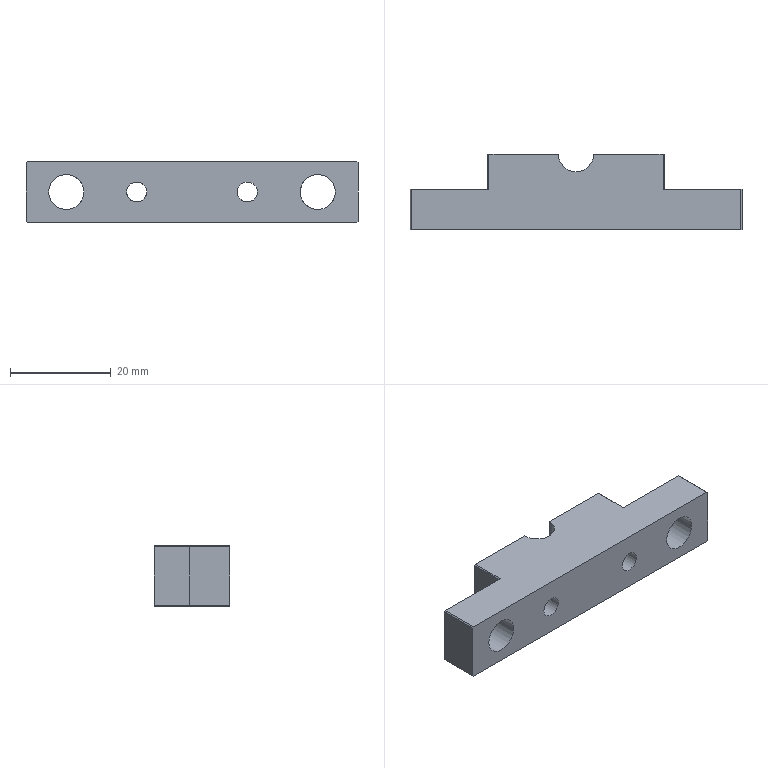CAM job | NX | 3+2 milling, drilling | part box 66 x 15 x 12 mm | stock box 73 x 19 x 19 mm
Tools:
number,name,description,diameter,corner_radius,flute_length,length,flutes
0,D4开粗,D4,4.0,0.0,12.0,50.0,2
2,D10开粗,D10,10.0,0.0,25.0,75.0,2
1,D63R0.8,方肩铣刀片,63.0,0.8,15.0,80.0,2
4,D8倒角刀,DJ8-32,8.0,0.0,4.0,60.0,2
8,R1,球头铣刀,2.0,1.0,4.0,4.0,2
6,Z3.3,Z3.3直柄钻头,3.3,0.0,36.0,65.0,2
0,M4X0.7,公制-铝用螺旋槽丝攻,3.3,0.0,13.0,21.0,2
5,D7钻头,Drilling Tool,7.0,0.0,35.0,50.0,2
Operations:
program,operation,operation_type,tool,method,geometry_group,spindle_rpm,surface_speed,feed_per_tooth,feed_cut,feed_plunge,cut_length_mm,path_length_mm,cut_time_min,machine_time_min
XX-CNC1,PLANAR_MILL,PlanarMilling,D10开粗,METHOD,MCS_1,4500.0,141.0,0.1111,1000.0,100.0,194.0,399.193,0.194,0.2145
XX-CNC1,ADAPTIVE_MILLING,CavityMilling,D10开粗,METHOD,W1,5500.0,100.0,0.1178,3000.0,100.0,393.878,479.878,0.1313,0.1399
XX-CNC1,PLANAR_MILL_1,PlanarMilling,D10开粗,METHOD,W1,4500.0,141.0,0.0889,800.0,100.0,598.841,878.456,0.7486,0.7765
XX-CNC1,PLANAR_MILL_1_COPY,PlanarMilling,D8倒角刀,METHOD,W1,4500.0,141.0,0.0889,800.0,100.0,177.725,237.725,0.2222,0.2282
XX-CNC1,DRILLING,Operation,D8倒角刀,METHOD,W1,3000.0,75.0,0.0333,200.0,0.0,13.0,139.09,0.065,0.0776
XX-CNC1,DRILLING_COPY,Operation,D8倒角刀,METHOD,W1,3000.0,75.0,0.0333,200.0,0.0,10.2,105.604,0.051,0.0605
XX-CNC1,PLANAR_MILL_COPY,PlanarMilling,D63R0.8,METHOD,MCS_1,3500.0,109.0,0.0857,600.0,100.0,150.0,206.0,0.25,0.2556
XX-CNC1,DRILLING_COPY_1,Operation,D7钻头,METHOD,W1,3000.0,75.0,0.0333,200.0,0.0,36.0,185.09,0.18,0.1949
XX-CNC1,HOLE_MILLING,CylinderMilling,D4开粗,METHOD,W1,4500.0,56.0,0.0222,200.0,100.0,28.274,234.274,0.1414,0.162
XX-CNC1,DRILLING_COPY_COPY,Operation,Z3.3,METHOD,W1,3000.0,75.0,0.0333,200.0,0.0,42.0,169.204,0.21,0.2227
XX-CNC1,DRILLING_COPY_COPY_COPY,Operation,M4X0.7,METHOD,W1,300.0,3.0,0.35,210.0,0.0,26.0,137.204,0.1238,0.1349
XX-CNC2,PLANAR_MILL_2,PlanarMilling,D10开粗,METHOD,MCS_2,4500.0,141.0,0.1111,1200.0,100.0,916.0,2187.89,0.7633,0.8905
XX-CNC2,PLANAR_MILL_2_COPY,PlanarMilling,D10开粗,METHOD,MCS_2,4500.0,141.0,0.0889,800.0,100.0,183.2,377.01,0.229,0.2484
XX-CNC2,PLANAR_MILL_3,PlanarMilling,D10开粗,METHOD,MCS_2,4500.0,100.0,0.1178,1200.0,100.0,947.861,1700.661,0.7899,0.8652
XX-CNC2,PLANAR_MILL_3_COPY,PlanarMilling,D10开粗,METHOD,MCS_2,4500.0,100.0,0.1178,800.0,100.0,189.824,407.824,0.2373,0.2591
XX-CNC2,PLANAR_MILL_3_COPY_COPY,PlanarMilling,D10开粗,METHOD,MCS_2,4500.0,100.0,0.1178,800.0,100.0,76.039,247.811,0.095,0.1122
XX-CNC2,DRILLING_1,Operation,D8倒角刀,METHOD,MCS_2,3000.0,0.0,0.0,200.0,0.0,10.2,105.604,0.051,0.0605
XX-CNC2,DRILLING_1_COPY,Operation,D8倒角刀,METHOD,MCS_2,3000.0,0.0,0.0,200.0,0.0,13.0,153.09,0.065,0.079
XX-CNC2,PLANAR_MILL_4,PlanarMilling,D8倒角刀,METHOD,MCS_2,3500.0,87.0,0.1429,1000.0,100.0,116.956,173.956,0.117,0.1227
XX-CNC2,CURVE_DRIVE,SurfaceContour,R1,METHOD,MCS_2,5500.0,34.0,0.1818,2000.0,100.0,1912.678,1967.228,0.9563,0.9618